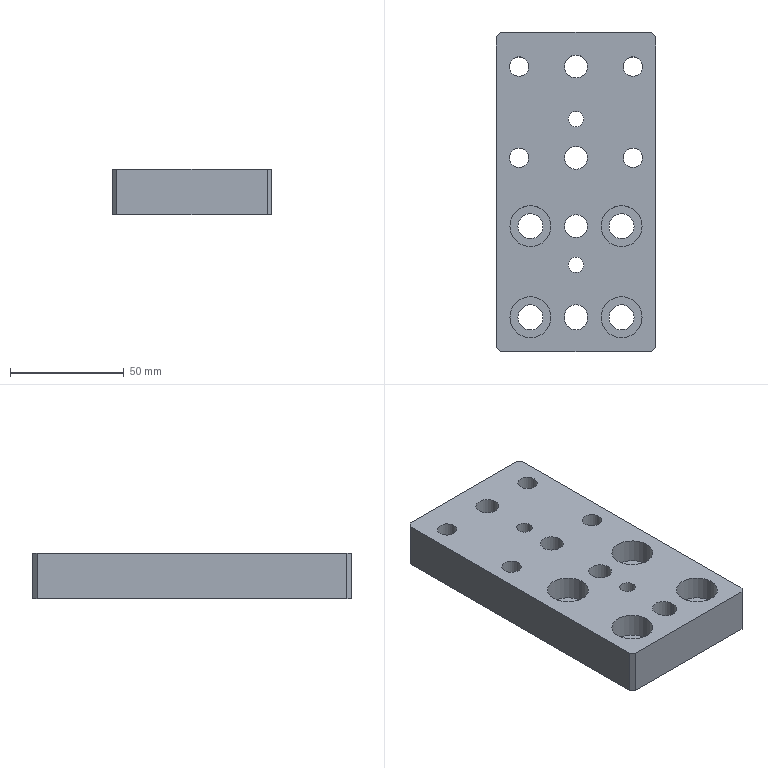Part | NX | 1 solid | 35 faces | box 70 x 140 x 20 mm | volume 169002 mm3 | cylinder 19 | plane 16 | commonest cylinder face diameters 10 x5 8.5 x4 11 x4 18 x4 6.8 x2
STEP:
#1=CARTESIAN_POINT('',(-33.,70.,10.));
#2=VERTEX_POINT('',#1);
#3=CARTESIAN_POINT('',(-35.,68.,10.));
#4=VERTEX_POINT('',#3);
#5=CARTESIAN_POINT('',(-51.5,51.5,10.));
#6=DIRECTION('',(-0.7071,-0.7071,0.));
#7=VECTOR('',#6,1000.);
#8=LINE('',#5,#7);
#9=EDGE_CURVE('',#2,#4,#8,.T.);
#10=ORIENTED_EDGE('',*,*,#9,.F.);
#11=CARTESIAN_POINT('',(-33.,70.,-10.));
#12=VERTEX_POINT('',#11);
#13=CARTESIAN_POINT('',(-33.,70.,10.));
#14=DIRECTION('',(0.,0.,1.));
#15=VECTOR('',#14,1000.);
#16=LINE('',#13,#15);
#17=EDGE_CURVE('',#12,#2,#16,.T.);
#18=ORIENTED_EDGE('',*,*,#17,.F.);
#19=CARTESIAN_POINT('',(-35.,68.,-10.));
#20=VERTEX_POINT('',#19);
#21=CARTESIAN_POINT('',(-35.,68.,-10.));
#22=DIRECTION('',(0.7071,0.7071,0.));
#23=VECTOR('',#22,1000.);
#24=LINE('',#21,#23);
#25=EDGE_CURVE('',#20,#12,#24,.T.);
#26=ORIENTED_EDGE('',*,*,#25,.F.);
#27=CARTESIAN_POINT('',(-35.,68.,10.));
#28=DIRECTION('',(0.,0.,-1.));
#29=VECTOR('',#28,1000.);
#30=LINE('',#27,#29);
#31=EDGE_CURVE('',#4,#20,#30,.T.);
#32=ORIENTED_EDGE('',*,*,#31,.F.);
#33=EDGE_LOOP('',(#10,#18,#26,#32));
#34=FACE_BOUND('',#33,.T.);
#35=CARTESIAN_POINT('',(-35.,68.,10.));
#36=DIRECTION('',(0.7071,-0.7071,0.));
#37=DIRECTION('',(0.,0.,-1.));
#38=AXIS2_PLACEMENT_3D('',#35,#36,#37);
#39=PLANE('',#38);
#40=ADVANCED_FACE('',(#34),#39,.F.);
#41=CARTESIAN_POINT('',(-35.,-68.,10.));
#42=VERTEX_POINT('',#41);
#43=CARTESIAN_POINT('',(-33.,-70.,10.));
#44=VERTEX_POINT('',#43);
#45=CARTESIAN_POINT('',(-51.5,-51.5,10.));
#46=DIRECTION('',(0.7071,-0.7071,0.));
#47=VECTOR('',#46,1000.);
#48=LINE('',#45,#47);
#49=EDGE_CURVE('',#42,#44,#48,.T.);
#50=ORIENTED_EDGE('',*,*,#49,.F.);
#51=CARTESIAN_POINT('',(-35.,-68.,-10.));
#52=VERTEX_POINT('',#51);
#53=CARTESIAN_POINT('',(-35.,-68.,10.));
#54=DIRECTION('',(0.,0.,1.));
#55=VECTOR('',#54,1000.);
#56=LINE('',#53,#55);
#57=EDGE_CURVE('',#52,#42,#56,.T.);
#58=ORIENTED_EDGE('',*,*,#57,.F.);
#59=CARTESIAN_POINT('',(-33.,-70.,-10.));
#60=VERTEX_POINT('',#59);
#61=CARTESIAN_POINT('',(-33.,-70.,-10.));
#62=DIRECTION('',(-0.7071,0.7071,0.));
#63=VECTOR('',#62,1000.);
#64=LINE('',#61,#63);
#65=EDGE_CURVE('',#60,#52,#64,.T.);
#66=ORIENTED_EDGE('',*,*,#65,.F.);
#67=CARTESIAN_POINT('',(-33.,-70.,10.));
#68=DIRECTION('',(0.,0.,-1.));
#69=VECTOR('',#68,1000.);
#70=LINE('',#67,#69);
#71=EDGE_CURVE('',#44,#60,#70,.T.);
#72=ORIENTED_EDGE('',*,*,#71,.F.);
#73=EDGE_LOOP('',(#50,#58,#66,#72));
#74=FACE_BOUND('',#73,.T.);
#75=CARTESIAN_POINT('',(-33.,-70.,10.));
#76=DIRECTION('',(0.7071,0.7071,0.));
#77=DIRECTION('',(0.,0.,-1.));
#78=AXIS2_PLACEMENT_3D('',#75,#76,#77);
#79=PLANE('',#78);
#80=ADVANCED_FACE('',(#74),#79,.F.);
#81=CARTESIAN_POINT('',(33.,-70.,10.));
#82=VERTEX_POINT('',#81);
#83=CARTESIAN_POINT('',(35.,-68.,10.));
#84=VERTEX_POINT('',#83);
#85=CARTESIAN_POINT('',(51.5,-51.5,10.));
#86=DIRECTION('',(0.7071,0.7071,0.));
#87=VECTOR('',#86,1000.);
#88=LINE('',#85,#87);
#89=EDGE_CURVE('',#82,#84,#88,.T.);
#90=ORIENTED_EDGE('',*,*,#89,.F.);
#91=CARTESIAN_POINT('',(33.,-70.,-10.));
#92=VERTEX_POINT('',#91);
#93=CARTESIAN_POINT('',(33.,-70.,10.));
#94=DIRECTION('',(0.,0.,1.));
#95=VECTOR('',#94,1000.);
#96=LINE('',#93,#95);
#97=EDGE_CURVE('',#92,#82,#96,.T.);
#98=ORIENTED_EDGE('',*,*,#97,.F.);
#99=CARTESIAN_POINT('',(35.,-68.,-10.));
#100=VERTEX_POINT('',#99);
#101=CARTESIAN_POINT('',(35.,-68.,-10.));
#102=DIRECTION('',(-0.7071,-0.7071,0.));
#103=VECTOR('',#102,1000.);
#104=LINE('',#101,#103);
#105=EDGE_CURVE('',#100,#92,#104,.T.);
#106=ORIENTED_EDGE('',*,*,#105,.F.);
#107=CARTESIAN_POINT('',(35.,-68.,10.));
#108=DIRECTION('',(0.,0.,-1.));
#109=VECTOR('',#108,1000.);
#110=LINE('',#107,#109);
#111=EDGE_CURVE('',#84,#100,#110,.T.);
#112=ORIENTED_EDGE('',*,*,#111,.F.);
#113=EDGE_LOOP('',(#90,#98,#106,#112));
#114=FACE_BOUND('',#113,.T.);
#115=CARTESIAN_POINT('',(35.,-68.,10.));
#116=DIRECTION('',(-0.7071,0.7071,0.));
#117=DIRECTION('',(0.,0.,-1.));
#118=AXIS2_PLACEMENT_3D('',#115,#116,#117);
#119=PLANE('',#118);
#120=ADVANCED_FACE('',(#114),#119,.F.);
#121=CARTESIAN_POINT('',(35.,68.,10.));
#122=VERTEX_POINT('',#121);
#123=CARTESIAN_POINT('',(33.,70.,10.));
#124=VERTEX_POINT('',#123);
#125=CARTESIAN_POINT('',(51.5,51.5,10.));
#126=DIRECTION('',(-0.7071,0.7071,0.));
#127=VECTOR('',#126,1000.);
#128=LINE('',#125,#127);
#129=EDGE_CURVE('',#122,#124,#128,.T.);
#130=ORIENTED_EDGE('',*,*,#129,.F.);
#131=CARTESIAN_POINT('',(35.,68.,-10.));
#132=VERTEX_POINT('',#131);
#133=CARTESIAN_POINT('',(35.,68.,10.));
#134=DIRECTION('',(0.,0.,1.));
#135=VECTOR('',#134,1000.);
#136=LINE('',#133,#135);
#137=EDGE_CURVE('',#132,#122,#136,.T.);
#138=ORIENTED_EDGE('',*,*,#137,.F.);
#139=CARTESIAN_POINT('',(33.,70.,-10.));
#140=VERTEX_POINT('',#139);
#141=CARTESIAN_POINT('',(33.,70.,-10.));
#142=DIRECTION('',(0.7071,-0.7071,0.));
#143=VECTOR('',#142,1000.);
#144=LINE('',#141,#143);
#145=EDGE_CURVE('',#140,#132,#144,.T.);
#146=ORIENTED_EDGE('',*,*,#145,.F.);
#147=CARTESIAN_POINT('',(33.,70.,10.));
#148=DIRECTION('',(0.,0.,-1.));
#149=VECTOR('',#148,1000.);
#150=LINE('',#147,#149);
#151=EDGE_CURVE('',#124,#140,#150,.T.);
#152=ORIENTED_EDGE('',*,*,#151,.F.);
#153=EDGE_LOOP('',(#130,#138,#146,#152));
#154=FACE_BOUND('',#153,.T.);
#155=CARTESIAN_POINT('',(33.,70.,10.));
#156=DIRECTION('',(-0.7071,-0.7071,0.));
#157=DIRECTION('',(0.,0.,-1.));
#158=AXIS2_PLACEMENT_3D('',#155,#156,#157);
#159=PLANE('',#158);
#160=ADVANCED_FACE('',(#154),#159,.F.);
#161=CARTESIAN_POINT('',(5.,-54.5,10.));
#162=VERTEX_POINT('',#161);
#163=CARTESIAN_POINT('',(5.,-54.5,-10.));
#164=VERTEX_POINT('',#163);
#165=CARTESIAN_POINT('',(5.,-54.5,-10.));
#166=DIRECTION('',(0.,0.,-1.));
#167=VECTOR('',#166,1000.);
#168=LINE('',#165,#167);
#169=EDGE_CURVE('',#162,#164,#168,.T.);
#170=ORIENTED_EDGE('',*,*,#169,.T.);
#171=CARTESIAN_POINT('',(5.,-55.5,-10.));
#172=VERTEX_POINT('',#171);
#173=CARTESIAN_POINT('',(5.,-55.5,-10.));
#174=DIRECTION('',(0.,1.,0.));
#175=VECTOR('',#174,1000.);
#176=LINE('',#173,#175);
#177=EDGE_CURVE('',#172,#164,#176,.T.);
#178=ORIENTED_EDGE('',*,*,#177,.F.);
#179=CARTESIAN_POINT('',(5.,-55.5,10.));
#180=VERTEX_POINT('',#179);
#181=CARTESIAN_POINT('',(5.,-55.5,-10.));
#182=DIRECTION('',(0.,0.,-1.));
#183=VECTOR('',#182,1000.);
#184=LINE('',#181,#183);
#185=EDGE_CURVE('',#180,#172,#184,.T.);
#186=ORIENTED_EDGE('',*,*,#185,.F.);
#187=CARTESIAN_POINT('',(5.,-55.5,10.));
#188=DIRECTION('',(0.,1.,0.));
#189=VECTOR('',#188,1000.);
#190=LINE('',#187,#189);
#191=EDGE_CURVE('',#180,#162,#190,.T.);
#192=ORIENTED_EDGE('',*,*,#191,.T.);
#193=EDGE_LOOP('',(#170,#178,#186,#192));
#194=FACE_BOUND('',#193,.T.);
#195=CARTESIAN_POINT('',(5.,-55.5,-10.));
#196=DIRECTION('',(1.,0.,0.));
#197=DIRECTION('',(0.,0.,-1.));
#198=AXIS2_PLACEMENT_3D('',#195,#196,#197);
#199=PLANE('',#198);
#200=ADVANCED_FACE('',(#194),#199,.F.);
#201=CARTESIAN_POINT('',(-5.,-54.5,-10.));
#202=VERTEX_POINT('',#201);
#203=CARTESIAN_POINT('',(-5.,-54.5,10.));
#204=VERTEX_POINT('',#203);
#205=CARTESIAN_POINT('',(-5.,-54.5,10.));
#206=DIRECTION('',(0.,0.,1.));
#207=VECTOR('',#206,1000.);
#208=LINE('',#205,#207);
#209=EDGE_CURVE('',#202,#204,#208,.T.);
#210=ORIENTED_EDGE('',*,*,#209,.T.);
#211=CARTESIAN_POINT('',(-5.,-55.5,10.));
#212=VERTEX_POINT('',#211);
#213=CARTESIAN_POINT('',(-5.,-55.5,10.));
#214=DIRECTION('',(0.,1.,0.));
#215=VECTOR('',#214,1000.);
#216=LINE('',#213,#215);
#217=EDGE_CURVE('',#212,#204,#216,.T.);
#218=ORIENTED_EDGE('',*,*,#217,.F.);
#219=CARTESIAN_POINT('',(-5.,-55.5,-10.));
#220=VERTEX_POINT('',#219);
#221=CARTESIAN_POINT('',(-5.,-55.5,10.));
#222=DIRECTION('',(0.,0.,-1.));
#223=VECTOR('',#222,1000.);
#224=LINE('',#221,#223);
#225=EDGE_CURVE('',#212,#220,#224,.T.);
#226=ORIENTED_EDGE('',*,*,#225,.T.);
#227=CARTESIAN_POINT('',(-5.,-55.5,-10.));
#228=DIRECTION('',(0.,1.,0.));
#229=VECTOR('',#228,1000.);
#230=LINE('',#227,#229);
#231=EDGE_CURVE('',#220,#202,#230,.T.);
#232=ORIENTED_EDGE('',*,*,#231,.T.);
#233=EDGE_LOOP('',(#210,#218,#226,#232));
#234=FACE_BOUND('',#233,.T.);
#235=CARTESIAN_POINT('',(-5.,-55.5,10.));
#236=DIRECTION('',(-1.,0.,0.));
#237=DIRECTION('',(0.,-1.,0.));
#238=AXIS2_PLACEMENT_3D('',#235,#236,#237);
#239=PLANE('',#238);
#240=ADVANCED_FACE('',(#234),#239,.F.);
#241=CARTESIAN_POINT('',(0.,-55.5,10.));
#242=DIRECTION('',(0.,0.,1.));
#243=DIRECTION('',(1.,0.,0.));
#244=AXIS2_PLACEMENT_3D('',#241,#242,#243);
#245=CIRCLE('',#244,5.);
#246=EDGE_CURVE('',#212,#180,#245,.T.);
#247=ORIENTED_EDGE('',*,*,#246,.T.);
#248=ORIENTED_EDGE('',*,*,#185,.T.);
#249=CARTESIAN_POINT('',(0.,-55.5,-10.));
#250=DIRECTION('',(0.,0.,1.));
#251=DIRECTION('',(1.,0.,0.));
#252=AXIS2_PLACEMENT_3D('',#249,#250,#251);
#253=CIRCLE('',#252,5.);
#254=EDGE_CURVE('',#220,#172,#253,.T.);
#255=ORIENTED_EDGE('',*,*,#254,.F.);
#256=ORIENTED_EDGE('',*,*,#225,.F.);
#257=EDGE_LOOP('',(#247,#248,#255,#256));
#258=FACE_BOUND('',#257,.T.);
#259=CARTESIAN_POINT('',(0.,-55.5,10.));
#260=DIRECTION('',(0.,0.,1.));
#261=DIRECTION('',(1.,0.,0.));
#262=AXIS2_PLACEMENT_3D('',#259,#260,#261);
#263=CYLINDRICAL_SURFACE('',#262,5.);
#264=ADVANCED_FACE('',(#258),#263,.F.);
#265=CARTESIAN_POINT('',(0.,-54.5,-10.));
#266=DIRECTION('',(0.,0.,1.));
#267=DIRECTION('',(1.,0.,0.));
#268=AXIS2_PLACEMENT_3D('',#265,#266,#267);
#269=CIRCLE('',#268,5.);
#270=EDGE_CURVE('',#164,#202,#269,.T.);
#271=ORIENTED_EDGE('',*,*,#270,.F.);
#272=ORIENTED_EDGE('',*,*,#169,.F.);
#273=CARTESIAN_POINT('',(0.,-54.5,10.));
#274=DIRECTION('',(0.,0.,1.));
#275=DIRECTION('',(1.,0.,0.));
#276=AXIS2_PLACEMENT_3D('',#273,#274,#275);
#277=CIRCLE('',#276,5.);
#278=EDGE_CURVE('',#162,#204,#277,.T.);
#279=ORIENTED_EDGE('',*,*,#278,.T.);
#280=ORIENTED_EDGE('',*,*,#209,.F.);
#281=EDGE_LOOP('',(#271,#272,#279,#280));
#282=FACE_BOUND('',#281,.T.);
#283=CARTESIAN_POINT('',(0.,-54.5,10.));
#284=DIRECTION('',(0.,0.,1.));
#285=DIRECTION('',(1.,0.,0.));
#286=AXIS2_PLACEMENT_3D('',#283,#284,#285);
#287=CYLINDRICAL_SURFACE('',#286,5.);
#288=ADVANCED_FACE('',(#282),#287,.F.);
#289=CARTESIAN_POINT('',(-11.,-55.,-0.6));
#290=VERTEX_POINT('',#289);
#291=CARTESIAN_POINT('',(-20.,-55.,-0.6));
#292=DIRECTION('',(0.,0.,1.));
#293=DIRECTION('',(1.,0.,0.));
#294=AXIS2_PLACEMENT_3D('',#291,#292,#293);
#295=CIRCLE('',#294,9.);
#296=EDGE_CURVE('',#290,#290,#295,.T.);
#297=ORIENTED_EDGE('',*,*,#296,.T.);
#298=EDGE_LOOP('',(#297));
#299=FACE_BOUND('',#298,.T.);
#300=CARTESIAN_POINT('',(-14.5,-55.,-0.6));
#301=VERTEX_POINT('',#300);
#302=CARTESIAN_POINT('',(-20.,-55.,-0.6));
#303=DIRECTION('',(0.,0.,1.));
#304=DIRECTION('',(1.,0.,0.));
#305=AXIS2_PLACEMENT_3D('',#302,#303,#304);
#306=CIRCLE('',#305,5.5);
#307=EDGE_CURVE('',#301,#301,#306,.T.);
#308=ORIENTED_EDGE('',*,*,#307,.F.);
#309=EDGE_LOOP('',(#308));
#310=FACE_BOUND('',#309,.T.);
#311=CARTESIAN_POINT('',(-14.5,-55.,-0.6));
#312=DIRECTION('',(0.,0.,-1.));
#313=DIRECTION('',(-1.,0.,0.));
#314=AXIS2_PLACEMENT_3D('',#311,#312,#313);
#315=PLANE('',#314);
#316=ADVANCED_FACE('',(#299,#310),#315,.F.);
#317=CARTESIAN_POINT('',(11.,-55.,-0.6));
#318=VERTEX_POINT('',#317);
#319=CARTESIAN_POINT('',(20.,-55.,-0.6));
#320=DIRECTION('',(0.,0.,1.));
#321=DIRECTION('',(-1.,0.,0.));
#322=AXIS2_PLACEMENT_3D('',#319,#320,#321);
#323=CIRCLE('',#322,9.);
#324=EDGE_CURVE('',#318,#318,#323,.T.);
#325=ORIENTED_EDGE('',*,*,#324,.T.);
#326=EDGE_LOOP('',(#325));
#327=FACE_BOUND('',#326,.T.);
#328=CARTESIAN_POINT('',(14.5,-55.,-0.6));
#329=VERTEX_POINT('',#328);
#330=CARTESIAN_POINT('',(20.,-55.,-0.6));
#331=DIRECTION('',(0.,0.,1.));
#332=DIRECTION('',(-1.,0.,0.));
#333=AXIS2_PLACEMENT_3D('',#330,#331,#332);
#334=CIRCLE('',#333,5.5);
#335=EDGE_CURVE('',#329,#329,#334,.T.);
#336=ORIENTED_EDGE('',*,*,#335,.F.);
#337=EDGE_LOOP('',(#336));
#338=FACE_BOUND('',#337,.T.);
#339=CARTESIAN_POINT('',(-14.5,-55.,-0.6));
#340=DIRECTION('',(0.,0.,-1.));
#341=DIRECTION('',(-1.,0.,0.));
#342=AXIS2_PLACEMENT_3D('',#339,#340,#341);
#343=PLANE('',#342);
#344=ADVANCED_FACE('',(#327,#338),#343,.F.);
#345=CARTESIAN_POINT('',(11.,-15.,-0.6));
#346=VERTEX_POINT('',#345);
#347=CARTESIAN_POINT('',(20.,-15.,-0.6));
#348=DIRECTION('',(0.,0.,1.));
#349=DIRECTION('',(-1.,0.,0.));
#350=AXIS2_PLACEMENT_3D('',#347,#348,#349);
#351=CIRCLE('',#350,9.);
#352=EDGE_CURVE('',#346,#346,#351,.T.);
#353=ORIENTED_EDGE('',*,*,#352,.T.);
#354=EDGE_LOOP('',(#353));
#355=FACE_BOUND('',#354,.T.);
#356=CARTESIAN_POINT('',(14.5,-15.,-0.6));
#357=VERTEX_POINT('',#356);
#358=CARTESIAN_POINT('',(20.,-15.,-0.6));
#359=DIRECTION('',(0.,0.,1.));
#360=DIRECTION('',(-1.,0.,0.));
#361=AXIS2_PLACEMENT_3D('',#358,#359,#360);
#362=CIRCLE('',#361,5.5);
#363=EDGE_CURVE('',#357,#357,#362,.T.);
#364=ORIENTED_EDGE('',*,*,#363,.F.);
#365=EDGE_LOOP('',(#364));
#366=FACE_BOUND('',#365,.T.);
#367=CARTESIAN_POINT('',(-14.5,-55.,-0.6));
#368=DIRECTION('',(0.,0.,-1.));
#369=DIRECTION('',(-1.,0.,0.));
#370=AXIS2_PLACEMENT_3D('',#367,#368,#369);
#371=PLANE('',#370);
#372=ADVANCED_FACE('',(#355,#366),#371,.F.);
#373=CARTESIAN_POINT('',(-29.,-15.,-0.6));
#374=VERTEX_POINT('',#373);
#375=CARTESIAN_POINT('',(-20.,-15.,-0.6));
#376=DIRECTION('',(0.,0.,1.));
#377=DIRECTION('',(-1.,0.,0.));
#378=AXIS2_PLACEMENT_3D('',#375,#376,#377);
#379=CIRCLE('',#378,9.);
#380=EDGE_CURVE('',#374,#374,#379,.T.);
#381=ORIENTED_EDGE('',*,*,#380,.T.);
#382=EDGE_LOOP('',(#381));
#383=FACE_BOUND('',#382,.T.);
#384=CARTESIAN_POINT('',(-25.5,-15.,-0.6));
#385=VERTEX_POINT('',#384);
#386=CARTESIAN_POINT('',(-20.,-15.,-0.6));
#387=DIRECTION('',(0.,0.,1.));
#388=DIRECTION('',(-1.,0.,0.));
#389=AXIS2_PLACEMENT_3D('',#386,#387,#388);
#390=CIRCLE('',#389,5.5);
#391=EDGE_CURVE('',#385,#385,#390,.T.);
#392=ORIENTED_EDGE('',*,*,#391,.F.);
#393=EDGE_LOOP('',(#392));
#394=FACE_BOUND('',#393,.T.);
#395=CARTESIAN_POINT('',(-14.5,-55.,-0.6));
#396=DIRECTION('',(0.,0.,-1.));
#397=DIRECTION('',(-1.,0.,0.));
#398=AXIS2_PLACEMENT_3D('',#395,#396,#397);
#399=PLANE('',#398);
#400=ADVANCED_FACE('',(#383,#394),#399,.F.);
#401=CARTESIAN_POINT('',(35.,70.,-10.));
#402=DIRECTION('',(-1.,0.,0.));
#403=VECTOR('',#402,1000.);
#404=LINE('',#401,#403);
#405=EDGE_CURVE('',#140,#12,#404,.T.);
#406=ORIENTED_EDGE('',*,*,#405,.F.);
#407=ORIENTED_EDGE('',*,*,#145,.T.);
#408=CARTESIAN_POINT('',(35.,-70.,-10.));
#409=DIRECTION('',(0.,1.,0.));
#410=VECTOR('',#409,1000.);
#411=LINE('',#408,#410);
#412=EDGE_CURVE('',#100,#132,#411,.T.);
#413=ORIENTED_EDGE('',*,*,#412,.F.);
#414=ORIENTED_EDGE('',*,*,#105,.T.);
#415=CARTESIAN_POINT('',(35.,-70.,-10.));
#416=DIRECTION('',(1.,0.,0.));
#417=VECTOR('',#416,1000.);
#418=LINE('',#415,#417);
#419=EDGE_CURVE('',#60,#92,#418,.T.);
#420=ORIENTED_EDGE('',*,*,#419,.F.);
#421=ORIENTED_EDGE('',*,*,#65,.T.);
#422=CARTESIAN_POINT('',(-35.,-70.,-10.));
#423=DIRECTION('',(0.,-1.,0.));
#424=VECTOR('',#423,1000.);
#425=LINE('',#422,#424);
#426=EDGE_CURVE('',#20,#52,#425,.T.);
#427=ORIENTED_EDGE('',*,*,#426,.F.);
#428=ORIENTED_EDGE('',*,*,#25,.T.);
#429=EDGE_LOOP('',(#406,#407,#413,#414,#420,#421,#427,#428));
#430=FACE_BOUND('',#429,.T.);
#431=CARTESIAN_POINT('',(-20.75,55.,-10.));
#432=VERTEX_POINT('',#431);
#433=CARTESIAN_POINT('',(-25.,55.,-10.));
#434=DIRECTION('',(0.,0.,1.));
#435=DIRECTION('',(1.,0.,0.));
#436=AXIS2_PLACEMENT_3D('',#433,#434,#435);
#437=CIRCLE('',#436,4.25);
#438=EDGE_CURVE('',#432,#432,#437,.T.);
#439=ORIENTED_EDGE('',*,*,#438,.T.);
#440=EDGE_LOOP('',(#439));
#441=FACE_BOUND('',#440,.T.);
#442=CARTESIAN_POINT('',(29.25,55.,-10.));
#443=VERTEX_POINT('',#442);
#444=CARTESIAN_POINT('',(25.,55.,-10.));
#445=DIRECTION('',(0.,0.,1.));
#446=DIRECTION('',(1.,0.,0.));
#447=AXIS2_PLACEMENT_3D('',#444,#445,#446);
#448=CIRCLE('',#447,4.25);
#449=EDGE_CURVE('',#443,#443,#448,.T.);
#450=ORIENTED_EDGE('',*,*,#449,.T.);
#451=EDGE_LOOP('',(#450));
#452=FACE_BOUND('',#451,.T.);
#453=CARTESIAN_POINT('',(29.25,15.,-10.));
#454=VERTEX_POINT('',#453);
#455=CARTESIAN_POINT('',(25.,15.,-10.));
#456=DIRECTION('',(0.,0.,1.));
#457=DIRECTION('',(1.,0.,0.));
#458=AXIS2_PLACEMENT_3D('',#455,#456,#457);
#459=CIRCLE('',#458,4.25);
#460=EDGE_CURVE('',#454,#454,#459,.T.);
#461=ORIENTED_EDGE('',*,*,#460,.T.);
#462=EDGE_LOOP('',(#461));
#463=FACE_BOUND('',#462,.T.);
#464=CARTESIAN_POINT('',(-20.75,15.,-10.));
#465=VERTEX_POINT('',#464);
#466=CARTESIAN_POINT('',(-25.,15.,-10.));
#467=DIRECTION('',(0.,0.,1.));
#468=DIRECTION('',(1.,0.,0.));
#469=AXIS2_PLACEMENT_3D('',#466,#467,#468);
#470=CIRCLE('',#469,4.25);
#471=EDGE_CURVE('',#465,#465,#470,.T.);
#472=ORIENTED_EDGE('',*,*,#471,.T.);
#473=EDGE_LOOP('',(#472));
#474=FACE_BOUND('',#473,.T.);
#475=CARTESIAN_POINT('',(5.,55.,-10.));
#476=VERTEX_POINT('',#475);
#477=CARTESIAN_POINT('',(0.,55.,-10.));
#478=DIRECTION('',(0.,0.,1.));
#479=DIRECTION('',(1.,0.,0.));
#480=AXIS2_PLACEMENT_3D('',#477,#478,#479);
#481=CIRCLE('',#480,5.);
#482=EDGE_CURVE('',#476,#476,#481,.T.);
#483=ORIENTED_EDGE('',*,*,#482,.T.);
#484=EDGE_LOOP('',(#483));
#485=FACE_BOUND('',#484,.T.);
#486=CARTESIAN_POINT('',(5.,15.,-10.));
#487=VERTEX_POINT('',#486);
#488=CARTESIAN_POINT('',(0.,15.,-10.));
#489=DIRECTION('',(0.,0.,1.));
#490=DIRECTION('',(1.,0.,0.));
#491=AXIS2_PLACEMENT_3D('',#488,#489,#490);
#492=CIRCLE('',#491,5.);
#493=EDGE_CURVE('',#487,#487,#492,.T.);
#494=ORIENTED_EDGE('',*,*,#493,.T.);
#495=EDGE_LOOP('',(#494));
#496=FACE_BOUND('',#495,.T.);
#497=CARTESIAN_POINT('',(-14.5,-15.,-10.));
#498=VERTEX_POINT('',#497);
#499=CARTESIAN_POINT('',(-20.,-15.,-10.));
#500=DIRECTION('',(0.,0.,1.));
#501=DIRECTION('',(1.,0.,0.));
#502=AXIS2_PLACEMENT_3D('',#499,#500,#501);
#503=CIRCLE('',#502,5.5);
#504=EDGE_CURVE('',#498,#498,#503,.T.);
#505=ORIENTED_EDGE('',*,*,#504,.T.);
#506=EDGE_LOOP('',(#505));
#507=FACE_BOUND('',#506,.T.);
#508=CARTESIAN_POINT('',(25.5,-15.,-10.));
#509=VERTEX_POINT('',#508);
#510=CARTESIAN_POINT('',(20.,-15.,-10.));
#511=DIRECTION('',(0.,0.,1.));
#512=DIRECTION('',(1.,0.,0.));
#513=AXIS2_PLACEMENT_3D('',#510,#511,#512);
#514=CIRCLE('',#513,5.5);
#515=EDGE_CURVE('',#509,#509,#514,.T.);
#516=ORIENTED_EDGE('',*,*,#515,.T.);
#517=EDGE_LOOP('',(#516));
#518=FACE_BOUND('',#517,.T.);
#519=CARTESIAN_POINT('',(25.5,-55.,-10.));
#520=VERTEX_POINT('',#519);
#521=CARTESIAN_POINT('',(20.,-55.,-10.));
#522=DIRECTION('',(0.,0.,1.));
#523=DIRECTION('',(1.,0.,0.));
#524=AXIS2_PLACEMENT_3D('',#521,#522,#523);
#525=CIRCLE('',#524,5.5);
#526=EDGE_CURVE('',#520,#520,#525,.T.);
#527=ORIENTED_EDGE('',*,*,#526,.T.);
#528=EDGE_LOOP('',(#527));
#529=FACE_BOUND('',#528,.T.);
#530=CARTESIAN_POINT('',(-14.5,-55.,-10.));
#531=VERTEX_POINT('',#530);
#532=CARTESIAN_POINT('',(-20.,-55.,-10.));
#533=DIRECTION('',(0.,0.,1.));
#534=DIRECTION('',(1.,0.,0.));
#535=AXIS2_PLACEMENT_3D('',#532,#533,#534);
#536=CIRCLE('',#535,5.5);
#537=EDGE_CURVE('',#531,#531,#536,.T.);
#538=ORIENTED_EDGE('',*,*,#537,.T.);
#539=EDGE_LOOP('',(#538));
#540=FACE_BOUND('',#539,.T.);
#541=CARTESIAN_POINT('',(5.,-15.,-10.));
#542=VERTEX_POINT('',#541);
#543=CARTESIAN_POINT('',(0.,-15.,-10.));
#544=DIRECTION('',(0.,0.,1.));
#545=DIRECTION('',(1.,0.,0.));
#546=AXIS2_PLACEMENT_3D('',#543,#544,#545);
#547=CIRCLE('',#546,5.);
#548=EDGE_CURVE('',#542,#542,#547,.T.);
#549=ORIENTED_EDGE('',*,*,#548,.T.);
#550=EDGE_LOOP('',(#549));
#551=FACE_BOUND('',#550,.T.);
#552=ORIENTED_EDGE('',*,*,#231,.F.);
#553=ORIENTED_EDGE('',*,*,#254,.T.);
#554=ORIENTED_EDGE('',*,*,#177,.T.);
#555=ORIENTED_EDGE('',*,*,#270,.T.);
#556=EDGE_LOOP('',(#552,#553,#554,#555));
#557=FACE_BOUND('',#556,.T.);
#558=CARTESIAN_POINT('',(3.4,32.,-10.));
#559=VERTEX_POINT('',#558);
#560=CARTESIAN_POINT('',(0.,32.,-10.));
#561=DIRECTION('',(0.,0.,1.));
#562=DIRECTION('',(1.,0.,0.));
#563=AXIS2_PLACEMENT_3D('',#560,#561,#562);
#564=CIRCLE('',#563,3.4);
#565=EDGE_CURVE('',#559,#559,#564,.T.);
#566=ORIENTED_EDGE('',*,*,#565,.T.);
#567=EDGE_LOOP('',(#566));
#568=FACE_BOUND('',#567,.T.);
#569=CARTESIAN_POINT('',(3.4,-32.,-10.));
#570=VERTEX_POINT('',#569);
#571=CARTESIAN_POINT('',(0.,-32.,-10.));
#572=DIRECTION('',(0.,0.,1.));
#573=DIRECTION('',(1.,0.,0.));
#574=AXIS2_PLACEMENT_3D('',#571,#572,#573);
#575=CIRCLE('',#574,3.4);
#576=EDGE_CURVE('',#570,#570,#575,.T.);
#577=ORIENTED_EDGE('',*,*,#576,.T.);
#578=EDGE_LOOP('',(#577));
#579=FACE_BOUND('',#578,.T.);
#580=CARTESIAN_POINT('',(0.,0.,-10.));
#581=DIRECTION('',(0.,0.,1.));
#582=DIRECTION('',(1.,0.,0.));
#583=AXIS2_PLACEMENT_3D('',#580,#581,#582);
#584=PLANE('',#583);
#585=ADVANCED_FACE('',(#430,#441,#452,#463,#474,#485,#496,#507,#518,#529,#540,#551,#557,#568,#579),#584,.F.);
#586=CARTESIAN_POINT('',(35.,70.,10.));
#587=DIRECTION('',(-1.,0.,0.));
#588=VECTOR('',#587,1000.);
#589=LINE('',#586,#588);
#590=EDGE_CURVE('',#124,#2,#589,.T.);
#591=ORIENTED_EDGE('',*,*,#590,.F.);
#592=ORIENTED_EDGE('',*,*,#151,.T.);
#593=ORIENTED_EDGE('',*,*,#405,.T.);
#594=ORIENTED_EDGE('',*,*,#17,.T.);
#595=EDGE_LOOP('',(#591,#592,#593,#594));
#596=FACE_BOUND('',#595,.T.);
#597=CARTESIAN_POINT('',(35.,70.,10.));
#598=DIRECTION('',(0.,-1.,0.));
#599=DIRECTION('',(0.,0.,-1.));
#600=AXIS2_PLACEMENT_3D('',#597,#598,#599);
#601=PLANE('',#600);
#602=ADVANCED_FACE('',(#596),#601,.F.);
#603=ORIENTED_EDGE('',*,*,#412,.T.);
#604=ORIENTED_EDGE('',*,*,#137,.T.);
#605=CARTESIAN_POINT('',(35.,-70.,10.));
#606=DIRECTION('',(0.,1.,0.));
#607=VECTOR('',#606,1000.);
#608=LINE('',#605,#607);
#609=EDGE_CURVE('',#84,#122,#608,.T.);
#610=ORIENTED_EDGE('',*,*,#609,.F.);
#611=ORIENTED_EDGE('',*,*,#111,.T.);
#612=EDGE_LOOP('',(#603,#604,#610,#611));
#613=FACE_BOUND('',#612,.T.);
#614=CARTESIAN_POINT('',(35.,-70.,10.));
#615=DIRECTION('',(-1.,0.,0.));
#616=DIRECTION('',(0.,0.,1.));
#617=AXIS2_PLACEMENT_3D('',#614,#615,#616);
#618=PLANE('',#617);
#619=ADVANCED_FACE('',(#613),#618,.F.);
#620=ORIENTED_EDGE('',*,*,#419,.T.);
#621=ORIENTED_EDGE('',*,*,#97,.T.);
#622=CARTESIAN_POINT('',(35.,-70.,10.));
#623=DIRECTION('',(1.,0.,0.));
#624=VECTOR('',#623,1000.);
#625=LINE('',#622,#624);
#626=EDGE_CURVE('',#44,#82,#625,.T.);
#627=ORIENTED_EDGE('',*,*,#626,.F.);
#628=ORIENTED_EDGE('',*,*,#71,.T.);
#629=EDGE_LOOP('',(#620,#621,#627,#628));
#630=FACE_BOUND('',#629,.T.);
#631=CARTESIAN_POINT('',(35.,-70.,10.));
#632=DIRECTION('',(0.,1.,0.));
#633=DIRECTION('',(0.,0.,1.));
#634=AXIS2_PLACEMENT_3D('',#631,#632,#633);
#635=PLANE('',#634);
#636=ADVANCED_FACE('',(#630),#635,.F.);
#637=ORIENTED_EDGE('',*,*,#426,.T.);
#638=ORIENTED_EDGE('',*,*,#57,.T.);
#639=CARTESIAN_POINT('',(-35.,-70.,10.));
#640=DIRECTION('',(0.,-1.,0.));
#641=VECTOR('',#640,1000.);
#642=LINE('',#639,#641);
#643=EDGE_CURVE('',#4,#42,#642,.T.);
#644=ORIENTED_EDGE('',*,*,#643,.F.);
#645=ORIENTED_EDGE('',*,*,#31,.T.);
#646=EDGE_LOOP('',(#637,#638,#644,#645));
#647=FACE_BOUND('',#646,.T.);
#648=CARTESIAN_POINT('',(-35.,-70.,10.));
#649=DIRECTION('',(1.,0.,0.));
#650=DIRECTION('',(0.,0.,-1.));
#651=AXIS2_PLACEMENT_3D('',#648,#649,#650);
#652=PLANE('',#651);
#653=ADVANCED_FACE('',(#647),#652,.F.);
#654=ORIENTED_EDGE('',*,*,#246,.F.);
#655=ORIENTED_EDGE('',*,*,#217,.T.);
#656=ORIENTED_EDGE('',*,*,#278,.F.);
#657=ORIENTED_EDGE('',*,*,#191,.F.);
#658=EDGE_LOOP('',(#654,#655,#656,#657));
#659=FACE_BOUND('',#658,.T.);
#660=ORIENTED_EDGE('',*,*,#609,.T.);
#661=ORIENTED_EDGE('',*,*,#129,.T.);
#662=ORIENTED_EDGE('',*,*,#590,.T.);
#663=ORIENTED_EDGE('',*,*,#9,.T.);
#664=ORIENTED_EDGE('',*,*,#643,.T.);
#665=ORIENTED_EDGE('',*,*,#49,.T.);
#666=ORIENTED_EDGE('',*,*,#626,.T.);
#667=ORIENTED_EDGE('',*,*,#89,.T.);
#668=EDGE_LOOP('',(#660,#661,#662,#663,#664,#665,#666,#667));
#669=FACE_BOUND('',#668,.T.);
#670=CARTESIAN_POINT('',(-20.75,55.,10.));
#671=VERTEX_POINT('',#670);
#672=CARTESIAN_POINT('',(-25.,55.,10.));
#673=DIRECTION('',(0.,0.,1.));
#674=DIRECTION('',(1.,0.,0.));
#675=AXIS2_PLACEMENT_3D('',#672,#673,#674);
#676=CIRCLE('',#675,4.25);
#677=EDGE_CURVE('',#671,#671,#676,.T.);
#678=ORIENTED_EDGE('',*,*,#677,.F.);
#679=EDGE_LOOP('',(#678));
#680=FACE_BOUND('',#679,.T.);
#681=CARTESIAN_POINT('',(29.25,55.,10.));
#682=VERTEX_POINT('',#681);
#683=CARTESIAN_POINT('',(25.,55.,10.));
#684=DIRECTION('',(0.,0.,1.));
#685=DIRECTION('',(1.,0.,0.));
#686=AXIS2_PLACEMENT_3D('',#683,#684,#685);
#687=CIRCLE('',#686,4.25);
#688=EDGE_CURVE('',#682,#682,#687,.T.);
#689=ORIENTED_EDGE('',*,*,#688,.F.);
#690=EDGE_LOOP('',(#689));
#691=FACE_BOUND('',#690,.T.);
#692=CARTESIAN_POINT('',(29.25,15.,10.));
#693=VERTEX_POINT('',#692);
#694=CARTESIAN_POINT('',(25.,15.,10.));
#695=DIRECTION('',(0.,0.,1.));
#696=DIRECTION('',(1.,0.,0.));
#697=AXIS2_PLACEMENT_3D('',#694,#695,#696);
#698=CIRCLE('',#697,4.25);
#699=EDGE_CURVE('',#693,#693,#698,.T.);
#700=ORIENTED_EDGE('',*,*,#699,.F.);
#701=EDGE_LOOP('',(#700));
#702=FACE_BOUND('',#701,.T.);
#703=CARTESIAN_POINT('',(-20.75,15.,10.));
#704=VERTEX_POINT('',#703);
#705=CARTESIAN_POINT('',(-25.,15.,10.));
#706=DIRECTION('',(0.,0.,1.));
#707=DIRECTION('',(1.,0.,0.));
#708=AXIS2_PLACEMENT_3D('',#705,#706,#707);
#709=CIRCLE('',#708,4.25);
#710=EDGE_CURVE('',#704,#704,#709,.T.);
#711=ORIENTED_EDGE('',*,*,#710,.F.);
#712=EDGE_LOOP('',(#711));
#713=FACE_BOUND('',#712,.T.);
#714=CARTESIAN_POINT('',(5.,55.,10.));
#715=VERTEX_POINT('',#714);
#716=CARTESIAN_POINT('',(0.,55.,10.));
#717=DIRECTION('',(0.,0.,1.));
#718=DIRECTION('',(1.,0.,0.));
#719=AXIS2_PLACEMENT_3D('',#716,#717,#718);
#720=CIRCLE('',#719,5.);
#721=EDGE_CURVE('',#715,#715,#720,.T.);
#722=ORIENTED_EDGE('',*,*,#721,.F.);
#723=EDGE_LOOP('',(#722));
#724=FACE_BOUND('',#723,.T.);
#725=CARTESIAN_POINT('',(5.,15.,10.));
#726=VERTEX_POINT('',#725);
#727=CARTESIAN_POINT('',(0.,15.,10.));
#728=DIRECTION('',(0.,0.,1.));
#729=DIRECTION('',(1.,0.,0.));
#730=AXIS2_PLACEMENT_3D('',#727,#728,#729);
#731=CIRCLE('',#730,5.);
#732=EDGE_CURVE('',#726,#726,#731,.T.);
#733=ORIENTED_EDGE('',*,*,#732,.F.);
#734=EDGE_LOOP('',(#733));
#735=FACE_BOUND('',#734,.T.);
#736=CARTESIAN_POINT('',(-11.,-15.,10.));
#737=VERTEX_POINT('',#736);
#738=CARTESIAN_POINT('',(-20.,-15.,10.));
#739=DIRECTION('',(0.,0.,1.));
#740=DIRECTION('',(1.,0.,0.));
#741=AXIS2_PLACEMENT_3D('',#738,#739,#740);
#742=CIRCLE('',#741,9.);
#743=EDGE_CURVE('',#737,#737,#742,.T.);
#744=ORIENTED_EDGE('',*,*,#743,.F.);
#745=EDGE_LOOP('',(#744));
#746=FACE_BOUND('',#745,.T.);
#747=CARTESIAN_POINT('',(29.,-15.,10.));
#748=VERTEX_POINT('',#747);
#749=CARTESIAN_POINT('',(20.,-15.,10.));
#750=DIRECTION('',(0.,0.,1.));
#751=DIRECTION('',(1.,0.,0.));
#752=AXIS2_PLACEMENT_3D('',#749,#750,#751);
#753=CIRCLE('',#752,9.);
#754=EDGE_CURVE('',#748,#748,#753,.T.);
#755=ORIENTED_EDGE('',*,*,#754,.F.);
#756=EDGE_LOOP('',(#755));
#757=FACE_BOUND('',#756,.T.);
#758=CARTESIAN_POINT('',(29.,-55.,10.));
#759=VERTEX_POINT('',#758);
#760=CARTESIAN_POINT('',(20.,-55.,10.));
#761=DIRECTION('',(0.,0.,1.));
#762=DIRECTION('',(1.,0.,0.));
#763=AXIS2_PLACEMENT_3D('',#760,#761,#762);
#764=CIRCLE('',#763,9.);
#765=EDGE_CURVE('',#759,#759,#764,.T.);
#766=ORIENTED_EDGE('',*,*,#765,.F.);
#767=EDGE_LOOP('',(#766));
#768=FACE_BOUND('',#767,.T.);
#769=CARTESIAN_POINT('',(-11.,-55.,10.));
#770=VERTEX_POINT('',#769);
#771=CARTESIAN_POINT('',(-20.,-55.,10.));
#772=DIRECTION('',(0.,0.,1.));
#773=DIRECTION('',(1.,0.,0.));
#774=AXIS2_PLACEMENT_3D('',#771,#772,#773);
#775=CIRCLE('',#774,9.);
#776=EDGE_CURVE('',#770,#770,#775,.T.);
#777=ORIENTED_EDGE('',*,*,#776,.F.);
#778=EDGE_LOOP('',(#777));
#779=FACE_BOUND('',#778,.T.);
#780=CARTESIAN_POINT('',(5.,-15.,10.));
#781=VERTEX_POINT('',#780);
#782=CARTESIAN_POINT('',(0.,-15.,10.));
#783=DIRECTION('',(0.,0.,1.));
#784=DIRECTION('',(1.,0.,0.));
#785=AXIS2_PLACEMENT_3D('',#782,#783,#784);
#786=CIRCLE('',#785,5.);
#787=EDGE_CURVE('',#781,#781,#786,.T.);
#788=ORIENTED_EDGE('',*,*,#787,.F.);
#789=EDGE_LOOP('',(#788));
#790=FACE_BOUND('',#789,.T.);
#791=CARTESIAN_POINT('',(3.4,32.,10.));
#792=VERTEX_POINT('',#791);
#793=CARTESIAN_POINT('',(0.,32.,10.));
#794=DIRECTION('',(0.,0.,1.));
#795=DIRECTION('',(1.,0.,0.));
#796=AXIS2_PLACEMENT_3D('',#793,#794,#795);
#797=CIRCLE('',#796,3.4);
#798=EDGE_CURVE('',#792,#792,#797,.T.);
#799=ORIENTED_EDGE('',*,*,#798,.F.);
#800=EDGE_LOOP('',(#799));
#801=FACE_BOUND('',#800,.T.);
#802=CARTESIAN_POINT('',(3.4,-32.,10.));
#803=VERTEX_POINT('',#802);
#804=CARTESIAN_POINT('',(0.,-32.,10.));
#805=DIRECTION('',(0.,0.,1.));
#806=DIRECTION('',(1.,0.,0.));
#807=AXIS2_PLACEMENT_3D('',#804,#805,#806);
#808=CIRCLE('',#807,3.4);
#809=EDGE_CURVE('',#803,#803,#808,.T.);
#810=ORIENTED_EDGE('',*,*,#809,.F.);
#811=EDGE_LOOP('',(#810));
#812=FACE_BOUND('',#811,.T.);
#813=CARTESIAN_POINT('',(0.,0.,10.));
#814=DIRECTION('',(0.,0.,1.));
#815=DIRECTION('',(1.,0.,0.));
#816=AXIS2_PLACEMENT_3D('',#813,#814,#815);
#817=PLANE('',#816);
#818=ADVANCED_FACE('',(#659,#669,#680,#691,#702,#713,#724,#735,#746,#757,#768,#779,#790,#801,#812),#817,.T.);
#819=ORIENTED_EDGE('',*,*,#438,.F.);
#820=EDGE_LOOP('',(#819));
#821=FACE_BOUND('',#820,.T.);
#822=ORIENTED_EDGE('',*,*,#677,.T.);
#823=EDGE_LOOP('',(#822));
#824=FACE_BOUND('',#823,.T.);
#825=CARTESIAN_POINT('',(-25.,55.,10.));
#826=DIRECTION('',(0.,0.,1.));
#827=DIRECTION('',(1.,0.,0.));
#828=AXIS2_PLACEMENT_3D('',#825,#826,#827);
#829=CYLINDRICAL_SURFACE('',#828,4.25);
#830=ADVANCED_FACE('',(#821,#824),#829,.F.);
#831=ORIENTED_EDGE('',*,*,#449,.F.);
#832=EDGE_LOOP('',(#831));
#833=FACE_BOUND('',#832,.T.);
#834=ORIENTED_EDGE('',*,*,#688,.T.);
#835=EDGE_LOOP('',(#834));
#836=FACE_BOUND('',#835,.T.);
#837=CARTESIAN_POINT('',(25.,55.,10.));
#838=DIRECTION('',(0.,0.,1.));
#839=DIRECTION('',(1.,0.,0.));
#840=AXIS2_PLACEMENT_3D('',#837,#838,#839);
#841=CYLINDRICAL_SURFACE('',#840,4.25);
#842=ADVANCED_FACE('',(#833,#836),#841,.F.);
#843=ORIENTED_EDGE('',*,*,#460,.F.);
#844=EDGE_LOOP('',(#843));
#845=FACE_BOUND('',#844,.T.);
#846=ORIENTED_EDGE('',*,*,#699,.T.);
#847=EDGE_LOOP('',(#846));
#848=FACE_BOUND('',#847,.T.);
#849=CARTESIAN_POINT('',(25.,15.,10.));
#850=DIRECTION('',(0.,0.,1.));
#851=DIRECTION('',(1.,0.,0.));
#852=AXIS2_PLACEMENT_3D('',#849,#850,#851);
#853=CYLINDRICAL_SURFACE('',#852,4.25);
#854=ADVANCED_FACE('',(#845,#848),#853,.F.);
#855=ORIENTED_EDGE('',*,*,#471,.F.);
#856=EDGE_LOOP('',(#855));
#857=FACE_BOUND('',#856,.T.);
#858=ORIENTED_EDGE('',*,*,#710,.T.);
#859=EDGE_LOOP('',(#858));
#860=FACE_BOUND('',#859,.T.);
#861=CARTESIAN_POINT('',(-25.,15.,10.));
#862=DIRECTION('',(0.,0.,1.));
#863=DIRECTION('',(1.,0.,0.));
#864=AXIS2_PLACEMENT_3D('',#861,#862,#863);
#865=CYLINDRICAL_SURFACE('',#864,4.25);
#866=ADVANCED_FACE('',(#857,#860),#865,.F.);
#867=ORIENTED_EDGE('',*,*,#482,.F.);
#868=EDGE_LOOP('',(#867));
#869=FACE_BOUND('',#868,.T.);
#870=ORIENTED_EDGE('',*,*,#721,.T.);
#871=EDGE_LOOP('',(#870));
#872=FACE_BOUND('',#871,.T.);
#873=CARTESIAN_POINT('',(0.,55.,10.));
#874=DIRECTION('',(0.,0.,1.));
#875=DIRECTION('',(1.,0.,0.));
#876=AXIS2_PLACEMENT_3D('',#873,#874,#875);
#877=CYLINDRICAL_SURFACE('',#876,5.);
#878=ADVANCED_FACE('',(#869,#872),#877,.F.);
#879=ORIENTED_EDGE('',*,*,#493,.F.);
#880=EDGE_LOOP('',(#879));
#881=FACE_BOUND('',#880,.T.);
#882=ORIENTED_EDGE('',*,*,#732,.T.);
#883=EDGE_LOOP('',(#882));
#884=FACE_BOUND('',#883,.T.);
#885=CARTESIAN_POINT('',(0.,15.,10.));
#886=DIRECTION('',(0.,0.,1.));
#887=DIRECTION('',(1.,0.,0.));
#888=AXIS2_PLACEMENT_3D('',#885,#886,#887);
#889=CYLINDRICAL_SURFACE('',#888,5.);
#890=ADVANCED_FACE('',(#881,#884),#889,.F.);
#891=ORIENTED_EDGE('',*,*,#504,.F.);
#892=EDGE_LOOP('',(#891));
#893=FACE_BOUND('',#892,.T.);
#894=ORIENTED_EDGE('',*,*,#391,.T.);
#895=EDGE_LOOP('',(#894));
#896=FACE_BOUND('',#895,.T.);
#897=CARTESIAN_POINT('',(-20.,-15.,10.));
#898=DIRECTION('',(0.,0.,1.));
#899=DIRECTION('',(1.,0.,0.));
#900=AXIS2_PLACEMENT_3D('',#897,#898,#899);
#901=CYLINDRICAL_SURFACE('',#900,5.5);
#902=ADVANCED_FACE('',(#893,#896),#901,.F.);
#903=ORIENTED_EDGE('',*,*,#380,.F.);
#904=EDGE_LOOP('',(#903));
#905=FACE_BOUND('',#904,.T.);
#906=ORIENTED_EDGE('',*,*,#743,.T.);
#907=EDGE_LOOP('',(#906));
#908=FACE_BOUND('',#907,.T.);
#909=CARTESIAN_POINT('',(-20.,-15.,10.));
#910=DIRECTION('',(0.,0.,1.));
#911=DIRECTION('',(1.,0.,0.));
#912=AXIS2_PLACEMENT_3D('',#909,#910,#911);
#913=CYLINDRICAL_SURFACE('',#912,9.);
#914=ADVANCED_FACE('',(#905,#908),#913,.F.);
#915=ORIENTED_EDGE('',*,*,#515,.F.);
#916=EDGE_LOOP('',(#915));
#917=FACE_BOUND('',#916,.T.);
#918=ORIENTED_EDGE('',*,*,#363,.T.);
#919=EDGE_LOOP('',(#918));
#920=FACE_BOUND('',#919,.T.);
#921=CARTESIAN_POINT('',(20.,-15.,10.));
#922=DIRECTION('',(0.,0.,1.));
#923=DIRECTION('',(1.,0.,0.));
#924=AXIS2_PLACEMENT_3D('',#921,#922,#923);
#925=CYLINDRICAL_SURFACE('',#924,5.5);
#926=ADVANCED_FACE('',(#917,#920),#925,.F.);
#927=ORIENTED_EDGE('',*,*,#352,.F.);
#928=EDGE_LOOP('',(#927));
#929=FACE_BOUND('',#928,.T.);
#930=ORIENTED_EDGE('',*,*,#754,.T.);
#931=EDGE_LOOP('',(#930));
#932=FACE_BOUND('',#931,.T.);
#933=CARTESIAN_POINT('',(20.,-15.,10.));
#934=DIRECTION('',(0.,0.,1.));
#935=DIRECTION('',(1.,0.,0.));
#936=AXIS2_PLACEMENT_3D('',#933,#934,#935);
#937=CYLINDRICAL_SURFACE('',#936,9.);
#938=ADVANCED_FACE('',(#929,#932),#937,.F.);
#939=ORIENTED_EDGE('',*,*,#526,.F.);
#940=EDGE_LOOP('',(#939));
#941=FACE_BOUND('',#940,.T.);
#942=ORIENTED_EDGE('',*,*,#335,.T.);
#943=EDGE_LOOP('',(#942));
#944=FACE_BOUND('',#943,.T.);
#945=CARTESIAN_POINT('',(20.,-55.,10.));
#946=DIRECTION('',(0.,0.,1.));
#947=DIRECTION('',(1.,0.,0.));
#948=AXIS2_PLACEMENT_3D('',#945,#946,#947);
#949=CYLINDRICAL_SURFACE('',#948,5.5);
#950=ADVANCED_FACE('',(#941,#944),#949,.F.);
#951=ORIENTED_EDGE('',*,*,#324,.F.);
#952=EDGE_LOOP('',(#951));
#953=FACE_BOUND('',#952,.T.);
#954=ORIENTED_EDGE('',*,*,#765,.T.);
#955=EDGE_LOOP('',(#954));
#956=FACE_BOUND('',#955,.T.);
#957=CARTESIAN_POINT('',(20.,-55.,10.));
#958=DIRECTION('',(0.,0.,1.));
#959=DIRECTION('',(1.,0.,0.));
#960=AXIS2_PLACEMENT_3D('',#957,#958,#959);
#961=CYLINDRICAL_SURFACE('',#960,9.);
#962=ADVANCED_FACE('',(#953,#956),#961,.F.);
#963=ORIENTED_EDGE('',*,*,#537,.F.);
#964=EDGE_LOOP('',(#963));
#965=FACE_BOUND('',#964,.T.);
#966=ORIENTED_EDGE('',*,*,#307,.T.);
#967=EDGE_LOOP('',(#966));
#968=FACE_BOUND('',#967,.T.);
#969=CARTESIAN_POINT('',(-20.,-55.,10.));
#970=DIRECTION('',(0.,0.,1.));
#971=DIRECTION('',(1.,0.,0.));
#972=AXIS2_PLACEMENT_3D('',#969,#970,#971);
#973=CYLINDRICAL_SURFACE('',#972,5.5);
#974=ADVANCED_FACE('',(#965,#968),#973,.F.);
#975=ORIENTED_EDGE('',*,*,#296,.F.);
#976=EDGE_LOOP('',(#975));
#977=FACE_BOUND('',#976,.T.);
#978=ORIENTED_EDGE('',*,*,#776,.T.);
#979=EDGE_LOOP('',(#978));
#980=FACE_BOUND('',#979,.T.);
#981=CARTESIAN_POINT('',(-20.,-55.,10.));
#982=DIRECTION('',(0.,0.,1.));
#983=DIRECTION('',(1.,0.,0.));
#984=AXIS2_PLACEMENT_3D('',#981,#982,#983);
#985=CYLINDRICAL_SURFACE('',#984,9.);
#986=ADVANCED_FACE('',(#977,#980),#985,.F.);
#987=ORIENTED_EDGE('',*,*,#548,.F.);
#988=EDGE_LOOP('',(#987));
#989=FACE_BOUND('',#988,.T.);
#990=ORIENTED_EDGE('',*,*,#787,.T.);
#991=EDGE_LOOP('',(#990));
#992=FACE_BOUND('',#991,.T.);
#993=CARTESIAN_POINT('',(0.,-15.,10.));
#994=DIRECTION('',(0.,0.,1.));
#995=DIRECTION('',(1.,0.,0.));
#996=AXIS2_PLACEMENT_3D('',#993,#994,#995);
#997=CYLINDRICAL_SURFACE('',#996,5.);
#998=ADVANCED_FACE('',(#989,#992),#997,.F.);
#999=ORIENTED_EDGE('',*,*,#565,.F.);
#1000=EDGE_LOOP('',(#999));
#1001=FACE_BOUND('',#1000,.T.);
#1002=ORIENTED_EDGE('',*,*,#798,.T.);
#1003=EDGE_LOOP('',(#1002));
#1004=FACE_BOUND('',#1003,.T.);
#1005=CARTESIAN_POINT('',(0.,32.,10.));
#1006=DIRECTION('',(0.,0.,1.));
#1007=DIRECTION('',(1.,0.,0.));
#1008=AXIS2_PLACEMENT_3D('',#1005,#1006,#1007);
#1009=CYLINDRICAL_SURFACE('',#1008,3.4);
#1010=ADVANCED_FACE('',(#1001,#1004),#1009,.F.);
#1011=ORIENTED_EDGE('',*,*,#576,.F.);
#1012=EDGE_LOOP('',(#1011));
#1013=FACE_BOUND('',#1012,.T.);
#1014=ORIENTED_EDGE('',*,*,#809,.T.);
#1015=EDGE_LOOP('',(#1014));
#1016=FACE_BOUND('',#1015,.T.);
#1017=CARTESIAN_POINT('',(0.,-32.,10.));
#1018=DIRECTION('',(0.,0.,1.));
#1019=DIRECTION('',(1.,0.,0.));
#1020=AXIS2_PLACEMENT_3D('',#1017,#1018,#1019);
#1021=CYLINDRICAL_SURFACE('',#1020,3.4);
#1022=ADVANCED_FACE('',(#1013,#1016),#1021,.F.);
#1023=CLOSED_SHELL('',(#40,#80,#120,#160,#200,#240,#264,#288,#316,#344,#372,#400,#585,#602,#619,#636,#653,#818,#830,#842,#854,#866,#878,#890,#902,#914,#926,#938,#950,#962,#974,#986,#998,#1010,#1022));
#1024=MANIFOLD_SOLID_BREP('',#1023);
#1025=(LENGTH_UNIT()NAMED_UNIT(*)SI_UNIT(.MILLI.,.METRE.));
#1026=UNCERTAINTY_MEASURE_WITH_UNIT(LENGTH_MEASURE(0.00001),#1025,'','');
#1027=(NAMED_UNIT(*)PLANE_ANGLE_UNIT()SI_UNIT($,.RADIAN.));
#1028=(NAMED_UNIT(*)SI_UNIT($,.STERADIAN.)SOLID_ANGLE_UNIT());
#1029=(GEOMETRIC_REPRESENTATION_CONTEXT(3)GLOBAL_UNCERTAINTY_ASSIGNED_CONTEXT((#1026))GLOBAL_UNIT_ASSIGNED_CONTEXT((#1025,#1027,#1028))REPRESENTATION_CONTEXT('',''));
#1030=ADVANCED_BREP_SHAPE_REPRESENTATION('',(#1024),#1029);